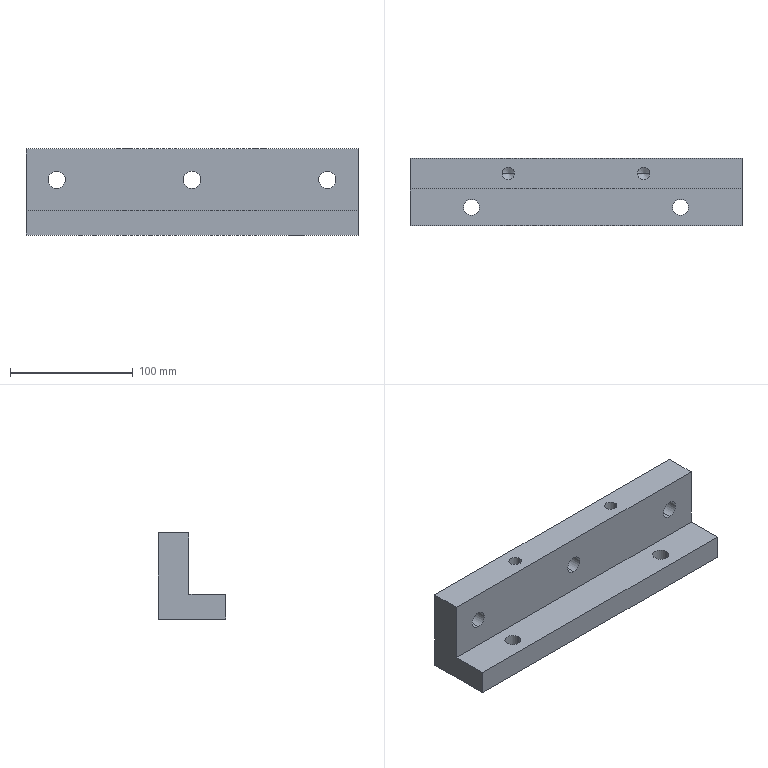Part | STEP file | CHAN DO MAT BAN GIUA | 1 solid | 26 faces | box 270 x 55 x 70 mm | volume 612670 mm3 | cylinder 14 | plane 8 | cone 4 | commonest cylinder face diameters 14 x6 10.106 x4 13 x4